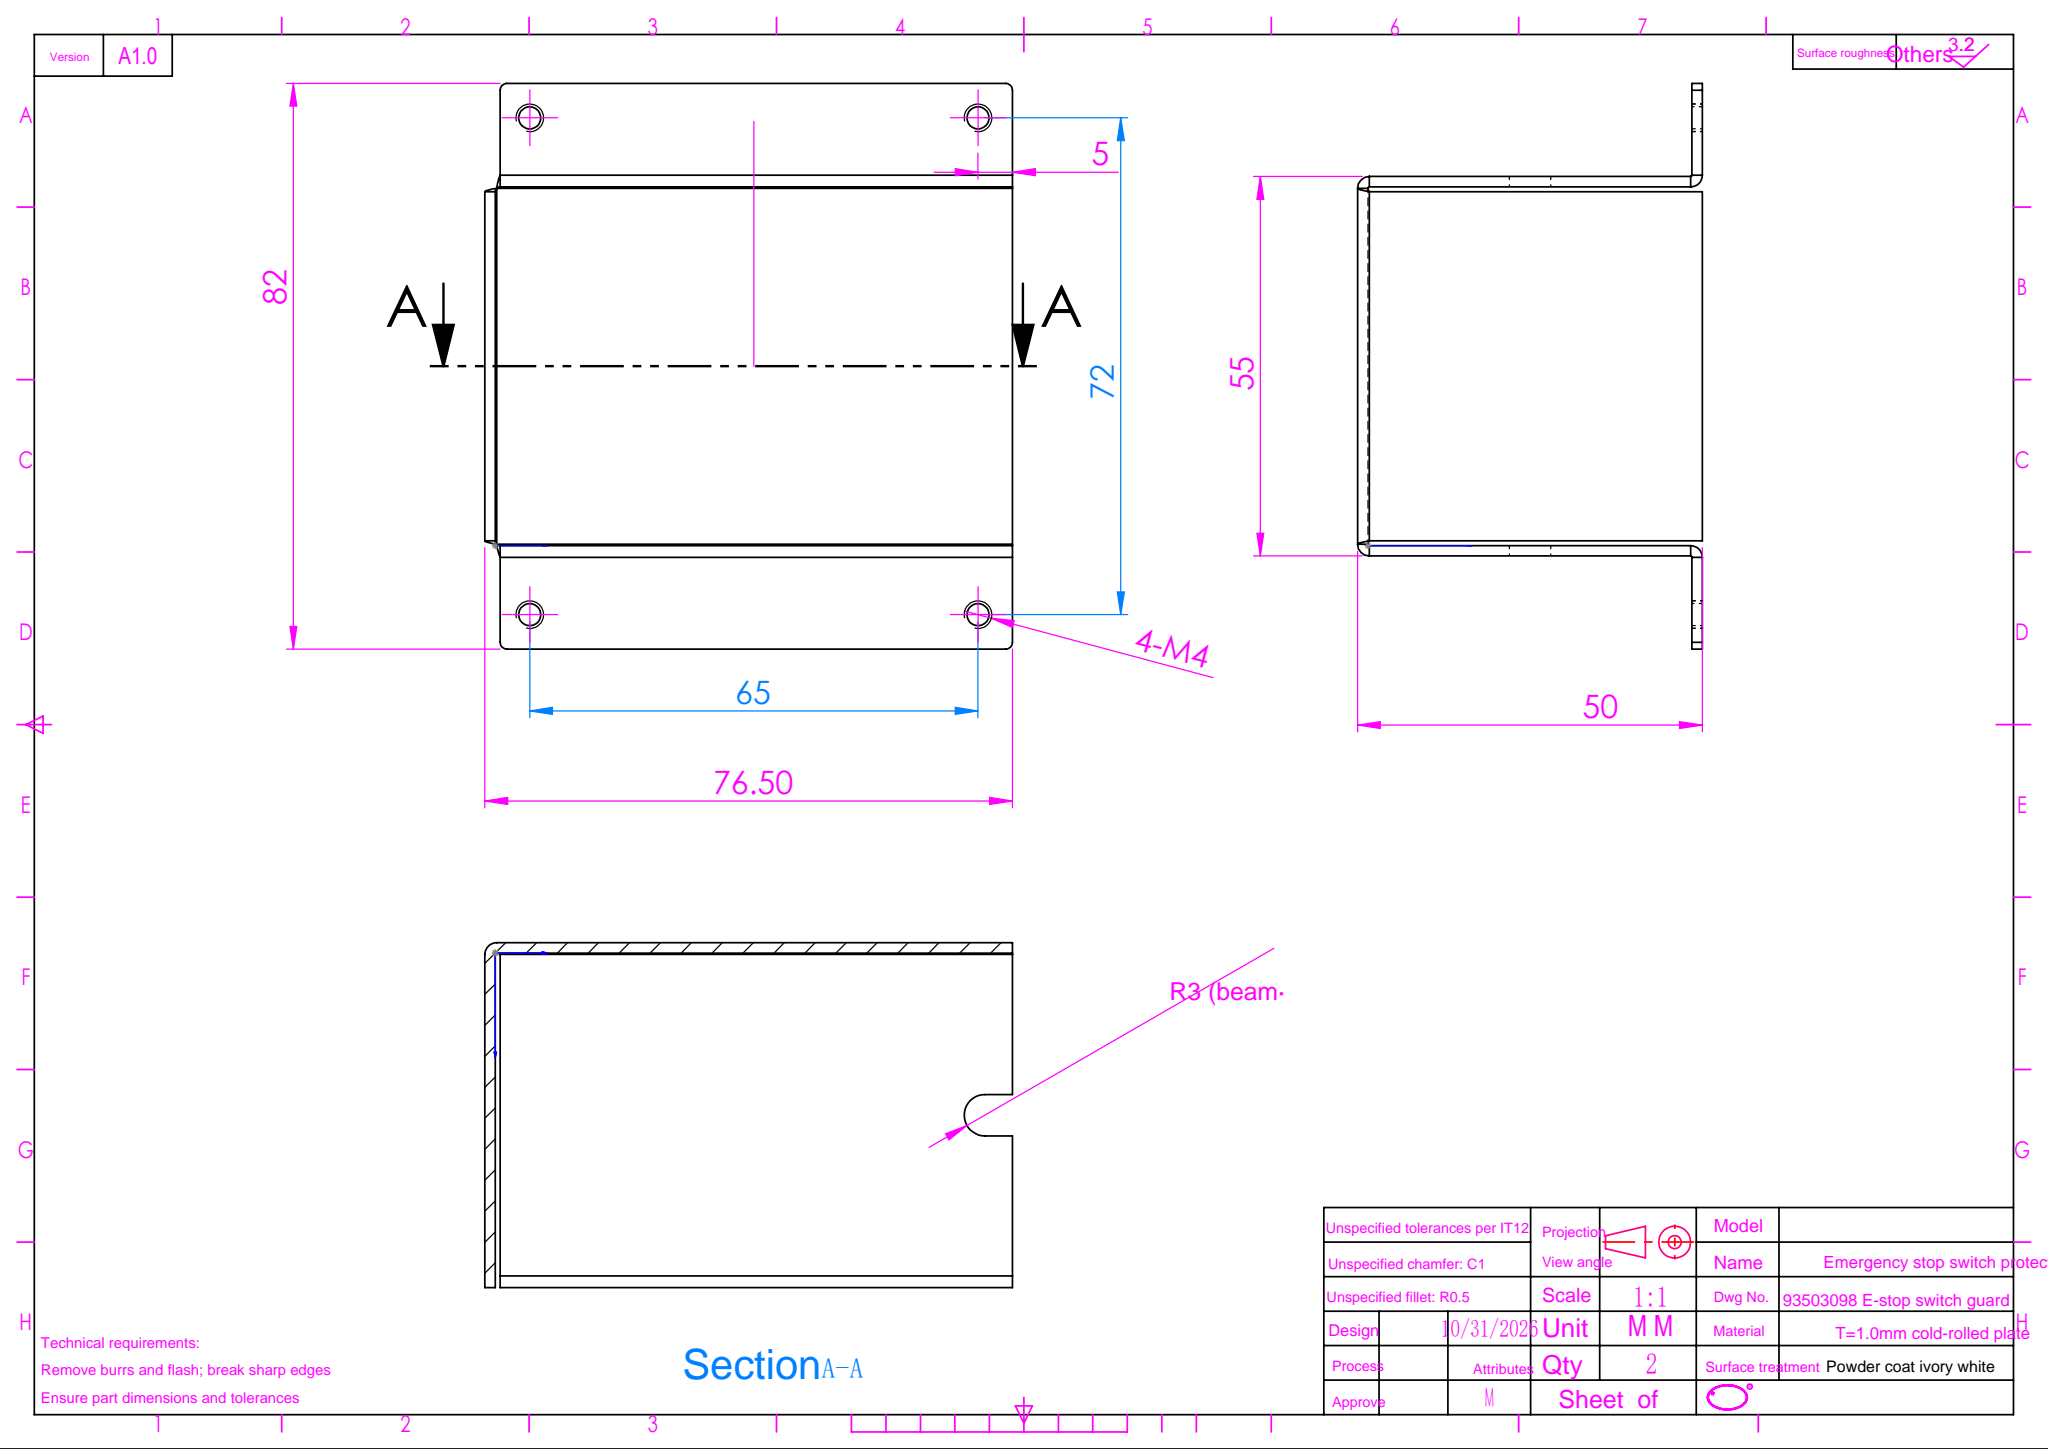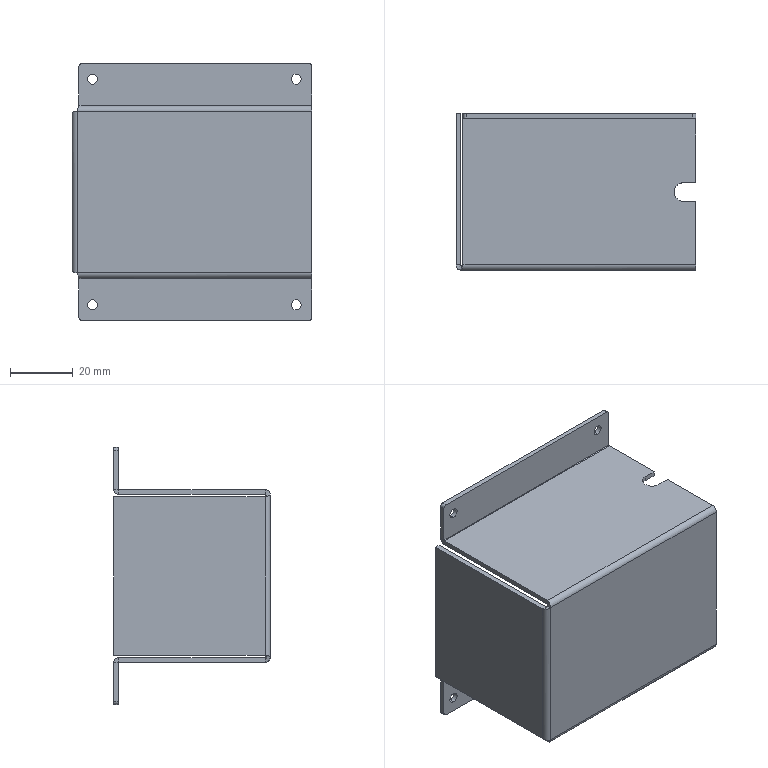Part | SolidWorks | features EdgeFlange 2, ICE 2, Fillet 1, FlatPattern 1, SMBaseFlange 1, SheetMetal 1 | 1 solid | 66 faces | box 76.5 x 50 x 82 mm | volume 23422 mm3 | plane 38 | cylinder 24 | spline 4 | commonest cylinder face diameters 3.2 x8 0.4 x5 3.4 x5 2 x4 6 x2